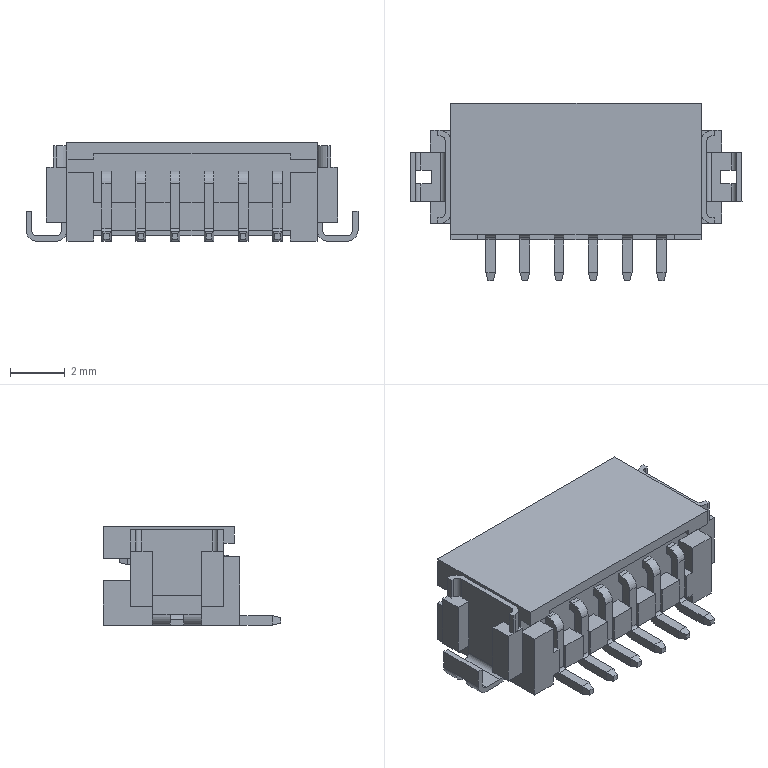Part | STEP file | RJ-USIO-V1_2-220411_197 | 1 solid | 350 faces | box 12.15 x 6.5 x 3.6 mm | volume 91.184 mm3 | plane 302 | cylinder 48 | commonest cylinder face diameters 0.4 x14 0.2 x12 0.9 x12 0.8 x10